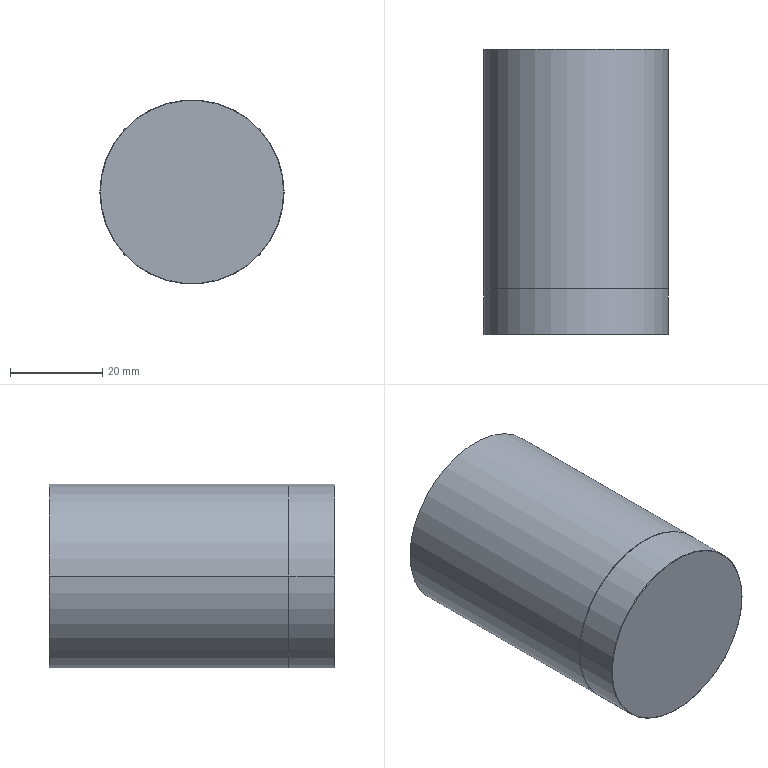Part | NX | 1 solid | 21 faces | box 40 x 61.99 x 40 mm | volume 26408 mm3 | cylinder 10 | cone 4 | plane 4 | torus 2 | sphere 1 | commonest cylinder face diameters 40 x4 10 x2 36 x2 39.7 x2
STEP:
#1=CARTESIAN_POINT('',(5.,-52.,0.));
#2=VERTEX_POINT('',#1);
#3=CARTESIAN_POINT('',(-5.,-52.,0.));
#4=VERTEX_POINT('',#3);
#5=CARTESIAN_POINT('',(0.,-52.,0.));
#6=DIRECTION('',(0.,1.,0.));
#7=DIRECTION('',(-1.,0.,0.));
#8=AXIS2_PLACEMENT_3D('',#5,#6,#7);
#9=CIRCLE('',#8,5.);
#10=EDGE_CURVE('',#2,#4,#9,.T.);
#11=ORIENTED_EDGE('',*,*,#10,.T.);
#12=CARTESIAN_POINT('',(-5.,-37.,0.));
#13=VERTEX_POINT('',#12);
#14=CARTESIAN_POINT('',(-5.,3.09,0.));
#15=DIRECTION('',(0.,-1.,0.));
#16=VECTOR('',#15,1000.);
#17=LINE('',#14,#16);
#18=EDGE_CURVE('',#4,#13,#17,.F.);
#19=ORIENTED_EDGE('',*,*,#18,.T.);
#20=CARTESIAN_POINT('',(5.,-37.,0.));
#21=VERTEX_POINT('',#20);
#22=CARTESIAN_POINT('',(0.,-37.,0.));
#23=DIRECTION('',(0.,1.,0.));
#24=DIRECTION('',(1.,0.,0.));
#25=AXIS2_PLACEMENT_3D('',#22,#23,#24);
#26=CIRCLE('',#25,5.);
#27=EDGE_CURVE('',#21,#13,#26,.T.);
#28=ORIENTED_EDGE('',*,*,#27,.F.);
#29=CARTESIAN_POINT('',(5.,3.09,0.));
#30=DIRECTION('',(0.,-1.,0.));
#31=VECTOR('',#30,1000.);
#32=LINE('',#29,#31);
#33=EDGE_CURVE('',#2,#21,#32,.F.);
#34=ORIENTED_EDGE('',*,*,#33,.F.);
#35=EDGE_LOOP('',(#11,#19,#28,#34));
#36=FACE_BOUND('',#35,.T.);
#37=CARTESIAN_POINT('',(0.,3.09,0.));
#38=DIRECTION('',(0.,-1.,0.));
#39=DIRECTION('',(-1.,0.,0.));
#40=AXIS2_PLACEMENT_3D('',#37,#38,#39);
#41=CYLINDRICAL_SURFACE('',#40,5.);
#42=ADVANCED_FACE('',(#36),#41,.T.);
#43=CARTESIAN_POINT('',(20.,-52.05,0.));
#44=VERTEX_POINT('',#43);
#45=CARTESIAN_POINT('',(-20.,-52.05,0.));
#46=VERTEX_POINT('',#45);
#47=CARTESIAN_POINT('',(0.,-52.05,0.));
#48=DIRECTION('',(0.,-1.,0.));
#49=DIRECTION('',(-1.,0.,0.));
#50=AXIS2_PLACEMENT_3D('',#47,#48,#49);
#51=CIRCLE('',#50,20.);
#52=EDGE_CURVE('',#44,#46,#51,.T.);
#53=ORIENTED_EDGE('',*,*,#52,.F.);
#54=CARTESIAN_POINT('',(19.95,-52.,0.));
#55=VERTEX_POINT('',#54);
#56=CARTESIAN_POINT('',(19.975,-52.025,0.));
#57=DIRECTION('',(0.7071,-0.7071,0.));
#58=VECTOR('',#57,1000.);
#59=LINE('',#56,#58);
#60=EDGE_CURVE('',#55,#44,#59,.T.);
#61=ORIENTED_EDGE('',*,*,#60,.F.);
#62=CARTESIAN_POINT('',(-19.95,-52.,0.));
#63=VERTEX_POINT('',#62);
#64=CARTESIAN_POINT('',(0.,-52.,0.));
#65=DIRECTION('',(0.,1.,0.));
#66=DIRECTION('',(-1.,0.,0.));
#67=AXIS2_PLACEMENT_3D('',#64,#65,#66);
#68=CIRCLE('',#67,19.95);
#69=EDGE_CURVE('',#63,#55,#68,.T.);
#70=ORIENTED_EDGE('',*,*,#69,.F.);
#71=CARTESIAN_POINT('',(-19.975,-52.025,0.));
#72=DIRECTION('',(-0.7071,-0.7071,0.));
#73=VECTOR('',#72,1000.);
#74=LINE('',#71,#73);
#75=EDGE_CURVE('',#63,#46,#74,.T.);
#76=ORIENTED_EDGE('',*,*,#75,.T.);
#77=EDGE_LOOP('',(#53,#61,#70,#76));
#78=FACE_BOUND('',#77,.T.);
#79=CARTESIAN_POINT('',(0.,-52.025,0.));
#80=DIRECTION('',(0.,-1.,0.));
#81=DIRECTION('',(-1.,0.,0.));
#82=AXIS2_PLACEMENT_3D('',#79,#80,#81);
#83=CONICAL_SURFACE('',#82,19.975,0.7854);
#84=ADVANCED_FACE('',(#78),#83,.T.);
#85=CARTESIAN_POINT('',(0.,-37.,0.));
#86=DIRECTION('',(0.,1.,0.));
#87=DIRECTION('',(1.,0.,0.));
#88=AXIS2_PLACEMENT_3D('',#85,#86,#87);
#89=CIRCLE('',#88,5.);
#90=EDGE_CURVE('',#13,#21,#89,.T.);
#91=ORIENTED_EDGE('',*,*,#90,.T.);
#92=ORIENTED_EDGE('',*,*,#27,.T.);
#93=EDGE_LOOP('',(#91,#92));
#94=FACE_BOUND('',#93,.T.);
#95=CARTESIAN_POINT('',(0.,-37.,0.));
#96=DIRECTION('',(0.,1.,0.));
#97=DIRECTION('',(1.,0.,0.));
#98=AXIS2_PLACEMENT_3D('',#95,#96,#97);
#99=SPHERICAL_SURFACE('',#98,5.);
#100=ADVANCED_FACE('',(#94),#99,.T.);
#101=CARTESIAN_POINT('',(20.,-61.9,0.));
#102=VERTEX_POINT('',#101);
#103=CARTESIAN_POINT('',(-20.,-61.9,0.));
#104=VERTEX_POINT('',#103);
#105=CARTESIAN_POINT('',(0.,-61.9,0.));
#106=DIRECTION('',(0.,1.,0.));
#107=DIRECTION('',(-1.,0.,0.));
#108=AXIS2_PLACEMENT_3D('',#105,#106,#107);
#109=CIRCLE('',#108,20.);
#110=EDGE_CURVE('',#102,#104,#109,.T.);
#111=ORIENTED_EDGE('',*,*,#110,.T.);
#112=CARTESIAN_POINT('',(-20.,3.09,0.));
#113=DIRECTION('',(0.,-1.,0.));
#114=VECTOR('',#113,1000.);
#115=LINE('',#112,#114);
#116=EDGE_CURVE('',#104,#46,#115,.F.);
#117=ORIENTED_EDGE('',*,*,#116,.T.);
#118=CARTESIAN_POINT('',(0.,-52.05,0.));
#119=DIRECTION('',(0.,-1.,0.));
#120=DIRECTION('',(-1.,0.,0.));
#121=AXIS2_PLACEMENT_3D('',#118,#119,#120);
#122=CIRCLE('',#121,20.);
#123=EDGE_CURVE('',#46,#44,#122,.T.);
#124=ORIENTED_EDGE('',*,*,#123,.T.);
#125=CARTESIAN_POINT('',(20.,3.09,0.));
#126=DIRECTION('',(0.,-1.,0.));
#127=VECTOR('',#126,1000.);
#128=LINE('',#125,#127);
#129=EDGE_CURVE('',#102,#44,#128,.F.);
#130=ORIENTED_EDGE('',*,*,#129,.F.);
#131=EDGE_LOOP('',(#111,#117,#124,#130));
#132=FACE_BOUND('',#131,.T.);
#133=CARTESIAN_POINT('',(0.,3.09,0.));
#134=DIRECTION('',(0.,-1.,0.));
#135=DIRECTION('',(-1.,0.,0.));
#136=AXIS2_PLACEMENT_3D('',#133,#134,#135);
#137=CYLINDRICAL_SURFACE('',#136,20.);
#138=ADVANCED_FACE('',(#132),#137,.T.);
#139=CARTESIAN_POINT('',(19.85,-52.,0.));
#140=VERTEX_POINT('',#139);
#141=CARTESIAN_POINT('',(-19.85,-52.,0.));
#142=VERTEX_POINT('',#141);
#143=CARTESIAN_POINT('',(0.,-52.,0.));
#144=DIRECTION('',(0.,-1.,0.));
#145=DIRECTION('',(1.,0.,0.));
#146=AXIS2_PLACEMENT_3D('',#143,#144,#145);
#147=CIRCLE('',#146,19.85);
#148=EDGE_CURVE('',#140,#142,#147,.T.);
#149=ORIENTED_EDGE('',*,*,#148,.F.);
#150=CARTESIAN_POINT('',(0.,-52.,0.));
#151=DIRECTION('',(0.,-1.,0.));
#152=DIRECTION('',(1.,0.,0.));
#153=AXIS2_PLACEMENT_3D('',#150,#151,#152);
#154=CIRCLE('',#153,19.85);
#155=EDGE_CURVE('',#142,#140,#154,.T.);
#156=ORIENTED_EDGE('',*,*,#155,.F.);
#157=EDGE_LOOP('',(#149,#156));
#158=FACE_BOUND('',#157,.T.);
#159=ORIENTED_EDGE('',*,*,#10,.F.);
#160=CARTESIAN_POINT('',(0.,-52.,0.));
#161=DIRECTION('',(0.,1.,0.));
#162=DIRECTION('',(-1.,0.,0.));
#163=AXIS2_PLACEMENT_3D('',#160,#161,#162);
#164=CIRCLE('',#163,5.);
#165=EDGE_CURVE('',#4,#2,#164,.T.);
#166=ORIENTED_EDGE('',*,*,#165,.F.);
#167=EDGE_LOOP('',(#159,#166));
#168=FACE_BOUND('',#167,.T.);
#169=CARTESIAN_POINT('',(0.,-52.,0.));
#170=DIRECTION('',(0.,-1.,0.));
#171=DIRECTION('',(0.,0.,-1.));
#172=AXIS2_PLACEMENT_3D('',#169,#170,#171);
#173=PLANE('',#172);
#174=ADVANCED_FACE('',(#158,#168),#173,.F.);
#175=ORIENTED_EDGE('',*,*,#148,.T.);
#176=CARTESIAN_POINT('',(-19.85,-51.95,0.));
#177=VERTEX_POINT('',#176);
#178=CARTESIAN_POINT('',(-19.85,3.09,0.));
#179=DIRECTION('',(0.,-1.,0.));
#180=VECTOR('',#179,1000.);
#181=LINE('',#178,#180);
#182=EDGE_CURVE('',#142,#177,#181,.F.);
#183=ORIENTED_EDGE('',*,*,#182,.T.);
#184=CARTESIAN_POINT('',(19.85,-51.95,0.));
#185=VERTEX_POINT('',#184);
#186=CARTESIAN_POINT('',(0.,-51.95,0.));
#187=DIRECTION('',(0.,1.,0.));
#188=DIRECTION('',(1.,0.,0.));
#189=AXIS2_PLACEMENT_3D('',#186,#187,#188);
#190=CIRCLE('',#189,19.85);
#191=EDGE_CURVE('',#177,#185,#190,.T.);
#192=ORIENTED_EDGE('',*,*,#191,.T.);
#193=CARTESIAN_POINT('',(19.85,3.09,0.));
#194=DIRECTION('',(0.,-1.,0.));
#195=VECTOR('',#194,1000.);
#196=LINE('',#193,#195);
#197=EDGE_CURVE('',#140,#185,#196,.F.);
#198=ORIENTED_EDGE('',*,*,#197,.F.);
#199=EDGE_LOOP('',(#175,#183,#192,#198));
#200=FACE_BOUND('',#199,.T.);
#201=CARTESIAN_POINT('',(0.,3.09,0.));
#202=DIRECTION('',(0.,-1.,0.));
#203=DIRECTION('',(-1.,0.,0.));
#204=AXIS2_PLACEMENT_3D('',#201,#202,#203);
#205=CYLINDRICAL_SURFACE('',#204,19.85);
#206=ADVANCED_FACE('',(#200),#205,.F.);
#207=ORIENTED_EDGE('',*,*,#110,.F.);
#208=CARTESIAN_POINT('',(19.9,-62.,0.));
#209=VERTEX_POINT('',#208);
#210=CARTESIAN_POINT('',(19.9,-61.9,0.));
#211=DIRECTION('',(0.,0.,1.));
#212=DIRECTION('',(1.,0.,0.));
#213=AXIS2_PLACEMENT_3D('',#210,#211,#212);
#214=CIRCLE('',#213,0.1);
#215=EDGE_CURVE('',#209,#102,#214,.T.);
#216=ORIENTED_EDGE('',*,*,#215,.F.);
#217=CARTESIAN_POINT('',(-19.9,-62.,0.));
#218=VERTEX_POINT('',#217);
#219=CARTESIAN_POINT('',(0.,-62.,0.));
#220=DIRECTION('',(0.,1.,0.));
#221=DIRECTION('',(1.,0.,0.));
#222=AXIS2_PLACEMENT_3D('',#219,#220,#221);
#223=CIRCLE('',#222,19.9);
#224=EDGE_CURVE('',#209,#218,#223,.T.);
#225=ORIENTED_EDGE('',*,*,#224,.T.);
#226=CARTESIAN_POINT('',(-19.9,-61.9,0.));
#227=DIRECTION('',(0.,0.,-1.));
#228=DIRECTION('',(-1.,0.,0.));
#229=AXIS2_PLACEMENT_3D('',#226,#227,#228);
#230=CIRCLE('',#229,0.1);
#231=EDGE_CURVE('',#218,#104,#230,.T.);
#232=ORIENTED_EDGE('',*,*,#231,.T.);
#233=EDGE_LOOP('',(#207,#216,#225,#232));
#234=FACE_BOUND('',#233,.T.);
#235=CARTESIAN_POINT('',(0.,-61.9,0.));
#236=DIRECTION('',(0.,-1.,0.));
#237=DIRECTION('',(-1.,0.,0.));
#238=AXIS2_PLACEMENT_3D('',#235,#236,#237);
#239=TOROIDAL_SURFACE('',#238,19.9,0.1);
#240=ADVANCED_FACE('',(#234),#239,.T.);
#241=ORIENTED_EDGE('',*,*,#191,.F.);
#242=CARTESIAN_POINT('',(0.,-51.95,0.));
#243=DIRECTION('',(0.,1.,0.));
#244=DIRECTION('',(1.,0.,0.));
#245=AXIS2_PLACEMENT_3D('',#242,#243,#244);
#246=CIRCLE('',#245,19.85);
#247=EDGE_CURVE('',#185,#177,#246,.T.);
#248=ORIENTED_EDGE('',*,*,#247,.F.);
#249=EDGE_LOOP('',(#241,#248));
#250=FACE_BOUND('',#249,.T.);
#251=CARTESIAN_POINT('',(-18.,-51.95,0.));
#252=VERTEX_POINT('',#251);
#253=CARTESIAN_POINT('',(18.,-51.95,0.));
#254=VERTEX_POINT('',#253);
#255=CARTESIAN_POINT('',(0.,-51.95,0.));
#256=DIRECTION('',(0.,-1.,0.));
#257=DIRECTION('',(1.,0.,0.));
#258=AXIS2_PLACEMENT_3D('',#255,#256,#257);
#259=CIRCLE('',#258,18.);
#260=EDGE_CURVE('',#252,#254,#259,.T.);
#261=ORIENTED_EDGE('',*,*,#260,.F.);
#262=CARTESIAN_POINT('',(0.,-51.95,0.));
#263=DIRECTION('',(0.,-1.,0.));
#264=DIRECTION('',(1.,0.,0.));
#265=AXIS2_PLACEMENT_3D('',#262,#263,#264);
#266=CIRCLE('',#265,18.);
#267=EDGE_CURVE('',#254,#252,#266,.T.);
#268=ORIENTED_EDGE('',*,*,#267,.F.);
#269=EDGE_LOOP('',(#261,#268));
#270=FACE_BOUND('',#269,.T.);
#271=CARTESIAN_POINT('',(0.,-51.95,0.));
#272=DIRECTION('',(0.,-1.,0.));
#273=DIRECTION('',(0.,0.,-1.));
#274=AXIS2_PLACEMENT_3D('',#271,#272,#273);
#275=PLANE('',#274);
#276=ADVANCED_FACE('',(#250,#270),#275,.T.);
#277=CARTESIAN_POINT('',(18.,-0.01,0.));
#278=VERTEX_POINT('',#277);
#279=CARTESIAN_POINT('',(-18.,-0.01,0.));
#280=VERTEX_POINT('',#279);
#281=CARTESIAN_POINT('',(0.,-0.01,0.));
#282=DIRECTION('',(0.,1.,0.));
#283=DIRECTION('',(1.,0.,0.));
#284=AXIS2_PLACEMENT_3D('',#281,#282,#283);
#285=CIRCLE('',#284,18.);
#286=EDGE_CURVE('',#278,#280,#285,.T.);
#287=ORIENTED_EDGE('',*,*,#286,.T.);
#288=CARTESIAN_POINT('',(-18.,3.09,0.));
#289=DIRECTION('',(0.,-1.,0.));
#290=VECTOR('',#289,1000.);
#291=LINE('',#288,#290);
#292=EDGE_CURVE('',#252,#280,#291,.F.);
#293=ORIENTED_EDGE('',*,*,#292,.F.);
#294=ORIENTED_EDGE('',*,*,#260,.T.);
#295=CARTESIAN_POINT('',(18.,3.09,0.));
#296=DIRECTION('',(0.,-1.,0.));
#297=VECTOR('',#296,1000.);
#298=LINE('',#295,#297);
#299=EDGE_CURVE('',#254,#278,#298,.F.);
#300=ORIENTED_EDGE('',*,*,#299,.T.);
#301=EDGE_LOOP('',(#287,#293,#294,#300));
#302=FACE_BOUND('',#301,.T.);
#303=CARTESIAN_POINT('',(0.,3.09,0.));
#304=DIRECTION('',(0.,-1.,0.));
#305=DIRECTION('',(-1.,0.,0.));
#306=AXIS2_PLACEMENT_3D('',#303,#304,#305);
#307=CYLINDRICAL_SURFACE('',#306,18.);
#308=ADVANCED_FACE('',(#302),#307,.F.);
#309=CARTESIAN_POINT('',(0.,-62.,0.));
#310=DIRECTION('',(0.,1.,0.));
#311=DIRECTION('',(1.,0.,0.));
#312=AXIS2_PLACEMENT_3D('',#309,#310,#311);
#313=CIRCLE('',#312,19.9);
#314=EDGE_CURVE('',#218,#209,#313,.T.);
#315=ORIENTED_EDGE('',*,*,#314,.F.);
#316=ORIENTED_EDGE('',*,*,#224,.F.);
#317=EDGE_LOOP('',(#315,#316));
#318=FACE_BOUND('',#317,.T.);
#319=CARTESIAN_POINT('',(0.,-62.,0.));
#320=DIRECTION('',(0.,-1.,0.));
#321=DIRECTION('',(0.,0.,-1.));
#322=AXIS2_PLACEMENT_3D('',#319,#320,#321);
#323=PLANE('',#322);
#324=ADVANCED_FACE('',(#318),#323,.T.);
#325=CARTESIAN_POINT('',(-20.,-0.01,0.));
#326=VERTEX_POINT('',#325);
#327=CARTESIAN_POINT('',(20.,-0.01,0.));
#328=VERTEX_POINT('',#327);
#329=CARTESIAN_POINT('',(0.,-0.01,0.));
#330=DIRECTION('',(0.,-1.,0.));
#331=DIRECTION('',(1.,0.,0.));
#332=AXIS2_PLACEMENT_3D('',#329,#330,#331);
#333=CIRCLE('',#332,20.);
#334=EDGE_CURVE('',#326,#328,#333,.T.);
#335=ORIENTED_EDGE('',*,*,#334,.F.);
#336=CARTESIAN_POINT('',(0.,-0.01,0.));
#337=DIRECTION('',(0.,-1.,0.));
#338=DIRECTION('',(1.,0.,0.));
#339=AXIS2_PLACEMENT_3D('',#336,#337,#338);
#340=CIRCLE('',#339,20.);
#341=EDGE_CURVE('',#328,#326,#340,.T.);
#342=ORIENTED_EDGE('',*,*,#341,.F.);
#343=EDGE_LOOP('',(#335,#342));
#344=FACE_BOUND('',#343,.T.);
#345=ORIENTED_EDGE('',*,*,#286,.F.);
#346=CARTESIAN_POINT('',(0.,-0.01,0.));
#347=DIRECTION('',(0.,1.,0.));
#348=DIRECTION('',(1.,0.,0.));
#349=AXIS2_PLACEMENT_3D('',#346,#347,#348);
#350=CIRCLE('',#349,18.);
#351=EDGE_CURVE('',#280,#278,#350,.T.);
#352=ORIENTED_EDGE('',*,*,#351,.F.);
#353=EDGE_LOOP('',(#345,#352));
#354=FACE_BOUND('',#353,.T.);
#355=CARTESIAN_POINT('',(0.,-0.01,0.));
#356=DIRECTION('',(0.,-1.,0.));
#357=DIRECTION('',(0.,0.,-1.));
#358=AXIS2_PLACEMENT_3D('',#355,#356,#357);
#359=PLANE('',#358);
#360=ADVANCED_FACE('',(#344,#354),#359,.F.);
#361=ORIENTED_EDGE('',*,*,#334,.T.);
#362=CARTESIAN_POINT('',(20.,-51.95,0.));
#363=VERTEX_POINT('',#362);
#364=CARTESIAN_POINT('',(20.,3.09,0.));
#365=DIRECTION('',(0.,-1.,0.));
#366=VECTOR('',#365,1000.);
#367=LINE('',#364,#366);
#368=EDGE_CURVE('',#328,#363,#367,.T.);
#369=ORIENTED_EDGE('',*,*,#368,.T.);
#370=CARTESIAN_POINT('',(-20.,-51.95,0.));
#371=VERTEX_POINT('',#370);
#372=CARTESIAN_POINT('',(0.,-51.95,0.));
#373=DIRECTION('',(0.,1.,0.));
#374=DIRECTION('',(1.,0.,0.));
#375=AXIS2_PLACEMENT_3D('',#372,#373,#374);
#376=CIRCLE('',#375,20.);
#377=EDGE_CURVE('',#363,#371,#376,.T.);
#378=ORIENTED_EDGE('',*,*,#377,.T.);
#379=CARTESIAN_POINT('',(-20.,3.09,0.));
#380=DIRECTION('',(0.,-1.,0.));
#381=VECTOR('',#380,1000.);
#382=LINE('',#379,#381);
#383=EDGE_CURVE('',#326,#371,#382,.T.);
#384=ORIENTED_EDGE('',*,*,#383,.F.);
#385=EDGE_LOOP('',(#361,#369,#378,#384));
#386=FACE_BOUND('',#385,.T.);
#387=CARTESIAN_POINT('',(0.,3.09,0.));
#388=DIRECTION('',(0.,-1.,0.));
#389=DIRECTION('',(-1.,0.,0.));
#390=AXIS2_PLACEMENT_3D('',#387,#388,#389);
#391=CYLINDRICAL_SURFACE('',#390,20.);
#392=ADVANCED_FACE('',(#386),#391,.T.);
#393=CARTESIAN_POINT('',(0.,-52.,0.));
#394=DIRECTION('',(0.,1.,0.));
#395=DIRECTION('',(-1.,0.,0.));
#396=AXIS2_PLACEMENT_3D('',#393,#394,#395);
#397=CIRCLE('',#396,19.95);
#398=EDGE_CURVE('',#55,#63,#397,.T.);
#399=ORIENTED_EDGE('',*,*,#398,.T.);
#400=CARTESIAN_POINT('',(-19.975,-51.975,0.));
#401=DIRECTION('',(-0.7071,0.7071,0.));
#402=VECTOR('',#401,1000.);
#403=LINE('',#400,#402);
#404=EDGE_CURVE('',#371,#63,#403,.F.);
#405=ORIENTED_EDGE('',*,*,#404,.F.);
#406=ORIENTED_EDGE('',*,*,#377,.F.);
#407=CARTESIAN_POINT('',(19.975,-51.975,0.));
#408=DIRECTION('',(0.7071,0.7071,0.));
#409=VECTOR('',#408,1000.);
#410=LINE('',#407,#409);
#411=EDGE_CURVE('',#363,#55,#410,.F.);
#412=ORIENTED_EDGE('',*,*,#411,.T.);
#413=EDGE_LOOP('',(#399,#405,#406,#412));
#414=FACE_BOUND('',#413,.T.);
#415=CARTESIAN_POINT('',(0.,-51.975,0.));
#416=DIRECTION('',(0.,1.,0.));
#417=DIRECTION('',(1.,0.,0.));
#418=AXIS2_PLACEMENT_3D('',#415,#416,#417);
#419=CONICAL_SURFACE('',#418,19.975,0.7854);
#420=ADVANCED_FACE('',(#414),#419,.T.);
#421=ORIENTED_EDGE('',*,*,#52,.T.);
#422=ORIENTED_EDGE('',*,*,#116,.F.);
#423=CARTESIAN_POINT('',(0.,-61.9,0.));
#424=DIRECTION('',(0.,1.,0.));
#425=DIRECTION('',(-1.,0.,0.));
#426=AXIS2_PLACEMENT_3D('',#423,#424,#425);
#427=CIRCLE('',#426,20.);
#428=EDGE_CURVE('',#104,#102,#427,.T.);
#429=ORIENTED_EDGE('',*,*,#428,.T.);
#430=ORIENTED_EDGE('',*,*,#129,.T.);
#431=EDGE_LOOP('',(#421,#422,#429,#430));
#432=FACE_BOUND('',#431,.T.);
#433=CARTESIAN_POINT('',(0.,3.09,0.));
#434=DIRECTION('',(0.,-1.,0.));
#435=DIRECTION('',(-1.,0.,0.));
#436=AXIS2_PLACEMENT_3D('',#433,#434,#435);
#437=CYLINDRICAL_SURFACE('',#436,20.);
#438=ADVANCED_FACE('',(#432),#437,.T.);
#439=CARTESIAN_POINT('',(0.,-51.95,0.));
#440=DIRECTION('',(0.,1.,0.));
#441=DIRECTION('',(1.,0.,0.));
#442=AXIS2_PLACEMENT_3D('',#439,#440,#441);
#443=CIRCLE('',#442,20.);
#444=EDGE_CURVE('',#371,#363,#443,.T.);
#445=ORIENTED_EDGE('',*,*,#444,.T.);
#446=ORIENTED_EDGE('',*,*,#368,.F.);
#447=ORIENTED_EDGE('',*,*,#341,.T.);
#448=ORIENTED_EDGE('',*,*,#383,.T.);
#449=EDGE_LOOP('',(#445,#446,#447,#448));
#450=FACE_BOUND('',#449,.T.);
#451=CARTESIAN_POINT('',(0.,3.09,0.));
#452=DIRECTION('',(0.,-1.,0.));
#453=DIRECTION('',(-1.,0.,0.));
#454=AXIS2_PLACEMENT_3D('',#451,#452,#453);
#455=CYLINDRICAL_SURFACE('',#454,20.);
#456=ADVANCED_FACE('',(#450),#455,.T.);
#457=ORIENTED_EDGE('',*,*,#90,.F.);
#458=ORIENTED_EDGE('',*,*,#18,.F.);
#459=ORIENTED_EDGE('',*,*,#165,.T.);
#460=ORIENTED_EDGE('',*,*,#33,.T.);
#461=EDGE_LOOP('',(#457,#458,#459,#460));
#462=FACE_BOUND('',#461,.T.);
#463=CARTESIAN_POINT('',(0.,3.09,0.));
#464=DIRECTION('',(0.,-1.,0.));
#465=DIRECTION('',(-1.,0.,0.));
#466=AXIS2_PLACEMENT_3D('',#463,#464,#465);
#467=CYLINDRICAL_SURFACE('',#466,5.);
#468=ADVANCED_FACE('',(#462),#467,.T.);
#469=ORIENTED_EDGE('',*,*,#444,.F.);
#470=ORIENTED_EDGE('',*,*,#404,.T.);
#471=ORIENTED_EDGE('',*,*,#69,.T.);
#472=ORIENTED_EDGE('',*,*,#411,.F.);
#473=EDGE_LOOP('',(#469,#470,#471,#472));
#474=FACE_BOUND('',#473,.T.);
#475=CARTESIAN_POINT('',(0.,-51.975,0.));
#476=DIRECTION('',(0.,1.,0.));
#477=DIRECTION('',(1.,0.,0.));
#478=AXIS2_PLACEMENT_3D('',#475,#476,#477);
#479=CONICAL_SURFACE('',#478,19.975,0.7854);
#480=ADVANCED_FACE('',(#474),#479,.T.);
#481=ORIENTED_EDGE('',*,*,#292,.T.);
#482=ORIENTED_EDGE('',*,*,#351,.T.);
#483=ORIENTED_EDGE('',*,*,#299,.F.);
#484=ORIENTED_EDGE('',*,*,#267,.T.);
#485=EDGE_LOOP('',(#481,#482,#483,#484));
#486=FACE_BOUND('',#485,.T.);
#487=CARTESIAN_POINT('',(0.,3.09,0.));
#488=DIRECTION('',(0.,-1.,0.));
#489=DIRECTION('',(-1.,0.,0.));
#490=AXIS2_PLACEMENT_3D('',#487,#488,#489);
#491=CYLINDRICAL_SURFACE('',#490,18.);
#492=ADVANCED_FACE('',(#486),#491,.F.);
#493=ORIENTED_EDGE('',*,*,#398,.F.);
#494=ORIENTED_EDGE('',*,*,#60,.T.);
#495=ORIENTED_EDGE('',*,*,#123,.F.);
#496=ORIENTED_EDGE('',*,*,#75,.F.);
#497=EDGE_LOOP('',(#493,#494,#495,#496));
#498=FACE_BOUND('',#497,.T.);
#499=CARTESIAN_POINT('',(0.,-52.025,0.));
#500=DIRECTION('',(0.,-1.,0.));
#501=DIRECTION('',(-1.,0.,0.));
#502=AXIS2_PLACEMENT_3D('',#499,#500,#501);
#503=CONICAL_SURFACE('',#502,19.975,0.7854);
#504=ADVANCED_FACE('',(#498),#503,.T.);
#505=ORIENTED_EDGE('',*,*,#182,.F.);
#506=ORIENTED_EDGE('',*,*,#155,.T.);
#507=ORIENTED_EDGE('',*,*,#197,.T.);
#508=ORIENTED_EDGE('',*,*,#247,.T.);
#509=EDGE_LOOP('',(#505,#506,#507,#508));
#510=FACE_BOUND('',#509,.T.);
#511=CARTESIAN_POINT('',(0.,3.09,0.));
#512=DIRECTION('',(0.,-1.,0.));
#513=DIRECTION('',(-1.,0.,0.));
#514=AXIS2_PLACEMENT_3D('',#511,#512,#513);
#515=CYLINDRICAL_SURFACE('',#514,19.85);
#516=ADVANCED_FACE('',(#510),#515,.F.);
#517=ORIENTED_EDGE('',*,*,#314,.T.);
#518=ORIENTED_EDGE('',*,*,#215,.T.);
#519=ORIENTED_EDGE('',*,*,#428,.F.);
#520=ORIENTED_EDGE('',*,*,#231,.F.);
#521=EDGE_LOOP('',(#517,#518,#519,#520));
#522=FACE_BOUND('',#521,.T.);
#523=CARTESIAN_POINT('',(0.,-61.9,0.));
#524=DIRECTION('',(0.,-1.,0.));
#525=DIRECTION('',(-1.,0.,0.));
#526=AXIS2_PLACEMENT_3D('',#523,#524,#525);
#527=TOROIDAL_SURFACE('',#526,19.9,0.1);
#528=ADVANCED_FACE('',(#522),#527,.T.);
#529=CLOSED_SHELL('',(#42,#84,#100,#138,#174,#206,#240,#276,#308,#324,#360,#392,#420,#438,#456,#468,#480,#492,#504,#516,#528));
#530=MANIFOLD_SOLID_BREP('',#529);
#531=(LENGTH_UNIT()NAMED_UNIT(*)SI_UNIT(.MILLI.,.METRE.));
#532=UNCERTAINTY_MEASURE_WITH_UNIT(LENGTH_MEASURE(0.00001),#531,'','');
#533=(NAMED_UNIT(*)PLANE_ANGLE_UNIT()SI_UNIT($,.RADIAN.));
#534=(NAMED_UNIT(*)SI_UNIT($,.STERADIAN.)SOLID_ANGLE_UNIT());
#535=(GEOMETRIC_REPRESENTATION_CONTEXT(3)GLOBAL_UNCERTAINTY_ASSIGNED_CONTEXT((#532))GLOBAL_UNIT_ASSIGNED_CONTEXT((#531,#533,#534))REPRESENTATION_CONTEXT('',''));
#536=ADVANCED_BREP_SHAPE_REPRESENTATION('',(#530),#535);